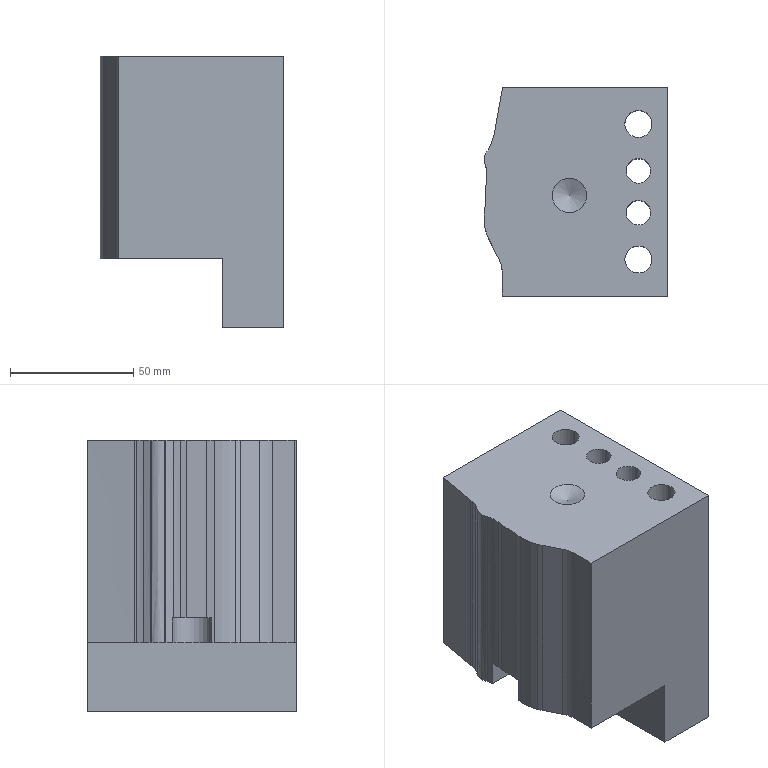Part | STEP file | PN_0046_id854_x_t | 1 solid | 45 faces | box 74.676 x 85 x 110 mm | volume 490062 mm3 | plane 18 | spline 13 | cylinder 10 | cone 4 | commonest cylinder face diameters 8.5 x2 10 x2 11 x2 17 x2 5.206 x1 16 x1